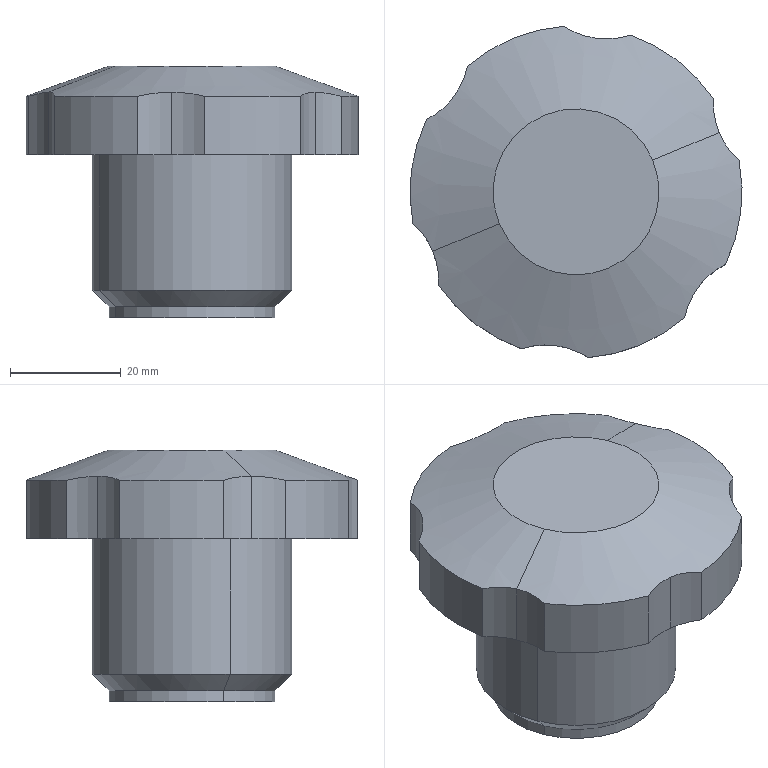Part | SolidWorks | features BaseBody 1 | 1 solid | 39 faces | box 60 x 59.84 x 45.5 mm | volume 53011 mm3 | cylinder 26 | plane 5 | cone 4 | torus 4 | commonest cylinder face diameters 28 x12 60 x6 20 x2 30 x2 36 x2 50 x2
STEP:
#1=CARTESIAN_POINT('',(32.407,459.424,549.15));
#2=VERTEX_POINT('',#1);
#3=CARTESIAN_POINT('',(78.593,478.576,549.15));
#4=VERTEX_POINT('',#3);
#5=CARTESIAN_POINT('',(55.5,469.,549.15));
#6=DIRECTION('',(0.,0.,1.));
#7=DIRECTION('',(-0.9237,-0.383,0.));
#8=AXIS2_PLACEMENT_3D('',#5,#6,#7);
#9=CIRCLE('',#8,25.);
#10=EDGE_CURVE('',#2,#4,#9,.T.);
#11=ORIENTED_EDGE('',*,*,#10,.T.);
#12=CARTESIAN_POINT('',(78.593,478.576,546.65));
#13=VERTEX_POINT('',#12);
#14=CARTESIAN_POINT('',(78.593,478.576,549.65));
#15=DIRECTION('',(0.,0.,-1.));
#16=VECTOR('',#15,1000.);
#17=LINE('',#14,#16);
#18=EDGE_CURVE('',#4,#13,#17,.T.);
#19=ORIENTED_EDGE('',*,*,#18,.T.);
#20=CARTESIAN_POINT('',(32.407,459.424,546.65));
#21=VERTEX_POINT('',#20);
#22=CARTESIAN_POINT('',(55.5,469.,546.65));
#23=DIRECTION('',(0.,0.,1.));
#24=DIRECTION('',(-0.9237,-0.383,0.));
#25=AXIS2_PLACEMENT_3D('',#22,#23,#24);
#26=CIRCLE('',#25,25.);
#27=EDGE_CURVE('',#21,#13,#26,.T.);
#28=ORIENTED_EDGE('',*,*,#27,.F.);
#29=CARTESIAN_POINT('',(32.407,459.424,549.65));
#30=DIRECTION('',(0.,0.,-1.));
#31=VECTOR('',#30,1000.);
#32=LINE('',#29,#31);
#33=EDGE_CURVE('',#2,#21,#32,.T.);
#34=ORIENTED_EDGE('',*,*,#33,.F.);
#35=EDGE_LOOP('',(#11,#19,#28,#34));
#36=FACE_OUTER_BOUND('',#35,.T.);
#37=CARTESIAN_POINT('',(55.5,469.,549.65));
#38=DIRECTION('',(0.,0.,-1.));
#39=DIRECTION('',(-0.9237,-0.383,0.));
#40=AXIS2_PLACEMENT_3D('',#37,#38,#39);
#41=CYLINDRICAL_SURFACE('',#40,25.);
#42=ADVANCED_FACE('',(#36),#41,.F.);
#43=CARTESIAN_POINT('',(38.873,462.105,549.15));
#44=VERTEX_POINT('',#43);
#45=CARTESIAN_POINT('',(72.127,475.895,549.15));
#46=VERTEX_POINT('',#45);
#47=CARTESIAN_POINT('',(55.5,469.,549.15));
#48=DIRECTION('',(0.,0.,-1.));
#49=DIRECTION('',(-0.9237,-0.383,0.));
#50=AXIS2_PLACEMENT_3D('',#47,#48,#49);
#51=CIRCLE('',#50,18.);
#52=EDGE_CURVE('',#44,#46,#51,.T.);
#53=ORIENTED_EDGE('',*,*,#52,.T.);
#54=CARTESIAN_POINT('',(72.127,475.895,522.15));
#55=VERTEX_POINT('',#54);
#56=CARTESIAN_POINT('',(72.127,475.895,549.65));
#57=DIRECTION('',(0.,0.,-1.));
#58=VECTOR('',#57,1000.);
#59=LINE('',#56,#58);
#60=EDGE_CURVE('',#46,#55,#59,.T.);
#61=ORIENTED_EDGE('',*,*,#60,.T.);
#62=CARTESIAN_POINT('',(38.873,462.105,522.15));
#63=VERTEX_POINT('',#62);
#64=CARTESIAN_POINT('',(55.5,469.,522.15));
#65=DIRECTION('',(0.,0.,1.));
#66=DIRECTION('',(0.9237,0.383,0.));
#67=AXIS2_PLACEMENT_3D('',#64,#65,#66);
#68=CIRCLE('',#67,18.);
#69=EDGE_CURVE('',#55,#63,#68,.T.);
#70=ORIENTED_EDGE('',*,*,#69,.T.);
#71=CARTESIAN_POINT('',(38.873,462.105,549.65));
#72=DIRECTION('',(0.,0.,-1.));
#73=VECTOR('',#72,1000.);
#74=LINE('',#71,#73);
#75=EDGE_CURVE('',#44,#63,#74,.T.);
#76=ORIENTED_EDGE('',*,*,#75,.F.);
#77=EDGE_LOOP('',(#53,#61,#70,#76));
#78=FACE_OUTER_BOUND('',#77,.T.);
#79=CARTESIAN_POINT('',(55.5,469.,549.65));
#80=DIRECTION('',(0.,0.,-1.));
#81=DIRECTION('',(-0.9237,-0.383,0.));
#82=AXIS2_PLACEMENT_3D('',#79,#80,#81);
#83=CYLINDRICAL_SURFACE('',#82,18.);
#84=ADVANCED_FACE('',(#78),#83,.T.);
#85=CARTESIAN_POINT('',(69.356,474.746,562.65));
#86=VERTEX_POINT('',#85);
#87=CARTESIAN_POINT('',(41.644,463.254,562.65));
#88=VERTEX_POINT('',#87);
#89=CARTESIAN_POINT('',(55.5,469.,562.65));
#90=DIRECTION('',(0.,0.,1.));
#91=DIRECTION('',(0.9237,0.383,0.));
#92=AXIS2_PLACEMENT_3D('',#89,#90,#91);
#93=CIRCLE('',#92,15.);
#94=EDGE_CURVE('',#86,#88,#93,.T.);
#95=ORIENTED_EDGE('',*,*,#94,.F.);
#96=CARTESIAN_POINT('',(81.364,479.725,557.918));
#97=VERTEX_POINT('',#96);
#98=CARTESIAN_POINT('',(83.212,480.491,557.19));
#99=DIRECTION('',(0.868,0.3599,-0.342));
#100=VECTOR('',#99,1000.);
#101=LINE('',#98,#100);
#102=EDGE_CURVE('',#86,#97,#101,.T.);
#103=ORIENTED_EDGE('',*,*,#102,.T.);
#104=CARTESIAN_POINT('',(80.318,485.855,557.19));
#105=VERTEX_POINT('',#104);
#106=CARTESIAN_POINT('',(80.318,485.855,557.19));
#107=CARTESIAN_POINT('',(80.261,484.818,557.419));
#108=CARTESIAN_POINT('',(80.318,483.785,557.601));
#109=CARTESIAN_POINT('',(80.536,482.496,557.757));
#110=CARTESIAN_POINT('',(80.587,482.239,557.785));
#111=CARTESIAN_POINT('',(80.704,481.724,557.833));
#112=CARTESIAN_POINT('',(80.77,481.467,557.854));
#113=CARTESIAN_POINT('',(80.99,480.705,557.902));
#114=CARTESIAN_POINT('',(81.164,480.21,557.918));
#115=CARTESIAN_POINT('',(81.364,479.725,557.918));
#116=B_SPLINE_CURVE_WITH_KNOTS('',3,(#106,#107,#108,#109,#110,#111,#112,#113,#114,#115),.UNSPECIFIED.,.F.,.F.,(4,2,2,2,4),(0.,0.003149,0.003936,0.004723,0.006297),.UNSPECIFIED.);
#117=EDGE_CURVE('',#105,#97,#116,.T.);
#118=ORIENTED_EDGE('',*,*,#117,.F.);
#119=CARTESIAN_POINT('',(65.335,497.342,557.19));
#120=VERTEX_POINT('',#119);
#121=CARTESIAN_POINT('',(55.5,469.,557.19));
#122=DIRECTION('',(0.,0.,-1.));
#123=DIRECTION('',(0.9237,0.383,0.));
#124=AXIS2_PLACEMENT_3D('',#121,#122,#123);
#125=CIRCLE('',#124,30.);
#126=EDGE_CURVE('',#120,#105,#125,.T.);
#127=ORIENTED_EDGE('',*,*,#126,.F.);
#128=CARTESIAN_POINT('',(59.144,496.762,557.918));
#129=VERTEX_POINT('',#128);
#130=CARTESIAN_POINT('',(59.144,496.762,557.918));
#131=CARTESIAN_POINT('',(59.663,496.694,557.918));
#132=CARTESIAN_POINT('',(60.186,496.655,557.902));
#133=CARTESIAN_POINT('',(61.239,496.636,557.838));
#134=CARTESIAN_POINT('',(61.771,496.656,557.789));
#135=CARTESIAN_POINT('',(63.335,496.805,557.601));
#136=CARTESIAN_POINT('',(64.349,497.018,557.419));
#137=CARTESIAN_POINT('',(65.335,497.342,557.19));
#138=B_SPLINE_CURVE_WITH_KNOTS('',3,(#130,#131,#132,#133,#134,#135,#136,#137),.UNSPECIFIED.,.F.,.F.,(4,2,2,4),(0.006297,0.007871,0.009445,0.01259),.UNSPECIFIED.);
#139=EDGE_CURVE('',#129,#120,#138,.T.);
#140=ORIENTED_EDGE('',*,*,#139,.F.);
#141=CARTESIAN_POINT('',(53.312,498.92,557.19));
#142=VERTEX_POINT('',#141);
#143=CARTESIAN_POINT('',(53.312,498.92,557.19));
#144=CARTESIAN_POINT('',(54.182,498.352,557.419));
#145=CARTESIAN_POINT('',(55.105,497.886,557.601));
#146=CARTESIAN_POINT('',(56.33,497.43,557.757));
#147=CARTESIAN_POINT('',(56.578,497.345,557.785));
#148=CARTESIAN_POINT('',(57.083,497.19,557.833));
#149=CARTESIAN_POINT('',(57.339,497.118,557.854));
#150=CARTESIAN_POINT('',(58.108,496.927,557.902));
#151=CARTESIAN_POINT('',(58.624,496.83,557.918));
#152=CARTESIAN_POINT('',(59.144,496.762,557.918));
#153=B_SPLINE_CURVE_WITH_KNOTS('',3,(#143,#144,#145,#146,#147,#148,#149,#150,#151,#152),.UNSPECIFIED.,.F.,.F.,(4,2,2,2,4),(0.,0.003149,0.003936,0.004723,0.006297),.UNSPECIFIED.);
#154=EDGE_CURVE('',#142,#129,#153,.T.);
#155=ORIENTED_EDGE('',*,*,#154,.F.);
#156=CARTESIAN_POINT('',(35.872,491.688,557.19));
#157=VERTEX_POINT('',#156);
#158=CARTESIAN_POINT('',(55.5,469.,557.19));
#159=DIRECTION('',(0.,0.,-1.));
#160=DIRECTION('',(0.9237,0.383,0.));
#161=AXIS2_PLACEMENT_3D('',#158,#159,#160);
#162=CIRCLE('',#161,30.);
#163=EDGE_CURVE('',#157,#142,#162,.T.);
#164=ORIENTED_EDGE('',*,*,#163,.F.);
#165=CARTESIAN_POINT('',(33.279,486.037,557.918));
#166=VERTEX_POINT('',#165);
#167=CARTESIAN_POINT('',(33.279,486.037,557.918));
#168=CARTESIAN_POINT('',(33.598,486.452,557.918));
#169=CARTESIAN_POINT('',(33.894,486.886,557.902));
#170=CARTESIAN_POINT('',(34.437,487.788,557.838));
#171=CARTESIAN_POINT('',(34.685,488.259,557.789));
#172=CARTESIAN_POINT('',(35.338,489.688,557.601));
#173=CARTESIAN_POINT('',(35.66,490.672,557.419));
#174=CARTESIAN_POINT('',(35.872,491.688,557.19));
#175=B_SPLINE_CURVE_WITH_KNOTS('',3,(#167,#168,#169,#170,#171,#172,#173,#174),.UNSPECIFIED.,.F.,.F.,(4,2,2,4),(0.006297,0.007871,0.009445,0.01259),.UNSPECIFIED.);
#176=EDGE_CURVE('',#166,#157,#175,.T.);
#177=ORIENTED_EDGE('',*,*,#176,.F.);
#178=CARTESIAN_POINT('',(28.494,482.065,557.19));
#179=VERTEX_POINT('',#178);
#180=CARTESIAN_POINT('',(28.494,482.065,557.19));
#181=CARTESIAN_POINT('',(29.421,482.534,557.419));
#182=CARTESIAN_POINT('',(30.287,483.101,557.601));
#183=CARTESIAN_POINT('',(31.294,483.934,557.757));
#184=CARTESIAN_POINT('',(31.491,484.107,557.785));
#185=CARTESIAN_POINT('',(31.878,484.465,557.833));
#186=CARTESIAN_POINT('',(32.068,484.652,557.854));
#187=CARTESIAN_POINT('',(32.618,485.222,557.902));
#188=CARTESIAN_POINT('',(32.96,485.621,557.918));
#189=CARTESIAN_POINT('',(33.279,486.037,557.918));
#190=B_SPLINE_CURVE_WITH_KNOTS('',3,(#180,#181,#182,#183,#184,#185,#186,#187,#188,#189),.UNSPECIFIED.,.F.,.F.,(4,2,2,2,4),(0.,0.003149,0.003936,0.004723,0.006297),.UNSPECIFIED.);
#191=EDGE_CURVE('',#179,#166,#190,.T.);
#192=ORIENTED_EDGE('',*,*,#191,.F.);
#193=CARTESIAN_POINT('',(26.038,463.346,557.19));
#194=VERTEX_POINT('',#193);
#195=CARTESIAN_POINT('',(55.5,469.,557.19));
#196=DIRECTION('',(0.,0.,-1.));
#197=DIRECTION('',(0.9237,0.383,0.));
#198=AXIS2_PLACEMENT_3D('',#195,#196,#197);
#199=CIRCLE('',#198,30.);
#200=EDGE_CURVE('',#194,#179,#199,.T.);
#201=ORIENTED_EDGE('',*,*,#200,.F.);
#202=CARTESIAN_POINT('',(29.636,458.275,557.918));
#203=VERTEX_POINT('',#202);
#204=CARTESIAN_POINT('',(29.636,458.275,557.918));
#205=CARTESIAN_POINT('',(29.435,458.759,557.918));
#206=CARTESIAN_POINT('',(29.207,459.231,557.902));
#207=CARTESIAN_POINT('',(28.697,460.153,557.838));
#208=CARTESIAN_POINT('',(28.413,460.603,557.789));
#209=CARTESIAN_POINT('',(27.502,461.883,557.601));
#210=CARTESIAN_POINT('',(26.811,462.654,557.419));
#211=CARTESIAN_POINT('',(26.038,463.346,557.19));
#212=B_SPLINE_CURVE_WITH_KNOTS('',3,(#204,#205,#206,#207,#208,#209,#210,#211),.UNSPECIFIED.,.F.,.F.,(4,2,2,4),(0.006297,0.007871,0.009445,0.01259),.UNSPECIFIED.);
#213=EDGE_CURVE('',#203,#194,#212,.T.);
#214=ORIENTED_EDGE('',*,*,#213,.F.);
#215=CARTESIAN_POINT('',(27.788,457.509,557.19));
#216=DIRECTION('',(-0.868,-0.3599,-0.342));
#217=VECTOR('',#216,1000.);
#218=LINE('',#215,#217);
#219=EDGE_CURVE('',#88,#203,#218,.T.);
#220=ORIENTED_EDGE('',*,*,#219,.F.);
#221=EDGE_LOOP('',(#95,#103,#118,#127,#140,#155,#164,#177,#192,#201,#214,#220));
#222=FACE_OUTER_BOUND('',#221,.T.);
#223=CARTESIAN_POINT('',(55.5,469.,557.19));
#224=DIRECTION('',(0.,0.,-1.));
#225=DIRECTION('',(-0.9237,-0.383,0.));
#226=AXIS2_PLACEMENT_3D('',#223,#224,#225);
#227=CONICAL_SURFACE('',#226,30.,1.222);
#228=ADVANCED_FACE('',(#222),#227,.T.);
#229=CARTESIAN_POINT('',(29.636,458.275,546.65));
#230=VERTEX_POINT('',#229);
#231=CARTESIAN_POINT('',(26.038,463.346,546.65));
#232=VERTEX_POINT('',#231);
#233=CARTESIAN_POINT('',(16.703,452.912,546.65));
#234=DIRECTION('',(0.,0.,1.));
#235=DIRECTION('',(-0.9237,-0.383,0.));
#236=AXIS2_PLACEMENT_3D('',#233,#234,#235);
#237=CIRCLE('',#236,14.);
#238=EDGE_CURVE('',#230,#232,#237,.T.);
#239=ORIENTED_EDGE('',*,*,#238,.F.);
#240=CARTESIAN_POINT('',(29.636,458.275,482.65));
#241=DIRECTION('',(0.,0.,1.));
#242=VECTOR('',#241,1000.);
#243=LINE('',#240,#242);
#244=EDGE_CURVE('',#230,#203,#243,.T.);
#245=ORIENTED_EDGE('',*,*,#244,.T.);
#246=ORIENTED_EDGE('',*,*,#213,.T.);
#247=CARTESIAN_POINT('',(26.038,463.346,551.92));
#248=DIRECTION('',(0.,0.,-1.));
#249=VECTOR('',#248,1000.);
#250=LINE('',#247,#249);
#251=EDGE_CURVE('',#194,#232,#250,.T.);
#252=ORIENTED_EDGE('',*,*,#251,.T.);
#253=EDGE_LOOP('',(#239,#245,#246,#252));
#254=FACE_OUTER_BOUND('',#253,.T.);
#255=CARTESIAN_POINT('',(16.703,452.912,482.65));
#256=DIRECTION('',(0.,0.,1.));
#257=DIRECTION('',(0.9237,0.383,0.));
#258=AXIS2_PLACEMENT_3D('',#255,#256,#257);
#259=CYLINDRICAL_SURFACE('',#258,14.);
#260=ADVANCED_FACE('',(#254),#259,.F.);
#261=CARTESIAN_POINT('',(51.856,441.238,546.65));
#262=VERTEX_POINT('',#261);
#263=CARTESIAN_POINT('',(45.665,440.658,546.65));
#264=VERTEX_POINT('',#263);
#265=CARTESIAN_POINT('',(50.034,427.357,546.65));
#266=DIRECTION('',(0.,0.,1.));
#267=DIRECTION('',(-0.9237,-0.383,0.));
#268=AXIS2_PLACEMENT_3D('',#265,#266,#267);
#269=CIRCLE('',#268,14.);
#270=EDGE_CURVE('',#262,#264,#269,.T.);
#271=ORIENTED_EDGE('',*,*,#270,.F.);
#272=CARTESIAN_POINT('',(51.856,441.238,557.918));
#273=VERTEX_POINT('',#272);
#274=CARTESIAN_POINT('',(51.856,441.238,482.65));
#275=DIRECTION('',(0.,0.,1.));
#276=VECTOR('',#275,1000.);
#277=LINE('',#274,#276);
#278=EDGE_CURVE('',#262,#273,#277,.T.);
#279=ORIENTED_EDGE('',*,*,#278,.T.);
#280=CARTESIAN_POINT('',(45.665,440.658,557.19));
#281=VERTEX_POINT('',#280);
#282=CARTESIAN_POINT('',(51.856,441.238,557.918));
#283=CARTESIAN_POINT('',(51.337,441.306,557.918));
#284=CARTESIAN_POINT('',(50.814,441.345,557.902));
#285=CARTESIAN_POINT('',(49.761,441.364,557.838));
#286=CARTESIAN_POINT('',(49.229,441.344,557.789));
#287=CARTESIAN_POINT('',(47.665,441.195,557.601));
#288=CARTESIAN_POINT('',(46.651,440.982,557.419));
#289=CARTESIAN_POINT('',(45.665,440.658,557.19));
#290=B_SPLINE_CURVE_WITH_KNOTS('',3,(#282,#283,#284,#285,#286,#287,#288,#289),.UNSPECIFIED.,.F.,.F.,(4,2,2,4),(0.006297,0.007871,0.009445,0.01259),.UNSPECIFIED.);
#291=EDGE_CURVE('',#273,#281,#290,.T.);
#292=ORIENTED_EDGE('',*,*,#291,.T.);
#293=CARTESIAN_POINT('',(45.665,440.658,551.92));
#294=DIRECTION('',(0.,0.,-1.));
#295=VECTOR('',#294,1000.);
#296=LINE('',#293,#295);
#297=EDGE_CURVE('',#281,#264,#296,.T.);
#298=ORIENTED_EDGE('',*,*,#297,.T.);
#299=EDGE_LOOP('',(#271,#279,#292,#298));
#300=FACE_OUTER_BOUND('',#299,.T.);
#301=CARTESIAN_POINT('',(50.034,427.357,482.65));
#302=DIRECTION('',(0.,0.,1.));
#303=DIRECTION('',(0.1301,0.9915,0.));
#304=AXIS2_PLACEMENT_3D('',#301,#302,#303);
#305=CYLINDRICAL_SURFACE('',#304,14.);
#306=ADVANCED_FACE('',(#300),#305,.F.);
#307=CARTESIAN_POINT('',(77.721,451.963,546.65));
#308=VERTEX_POINT('',#307);
#309=CARTESIAN_POINT('',(75.128,446.312,546.65));
#310=VERTEX_POINT('',#309);
#311=CARTESIAN_POINT('',(88.831,443.445,546.65));
#312=DIRECTION('',(0.,0.,1.));
#313=DIRECTION('',(-0.9237,-0.383,0.));
#314=AXIS2_PLACEMENT_3D('',#311,#312,#313);
#315=CIRCLE('',#314,14.);
#316=EDGE_CURVE('',#308,#310,#315,.T.);
#317=ORIENTED_EDGE('',*,*,#316,.F.);
#318=CARTESIAN_POINT('',(77.721,451.963,557.918));
#319=VERTEX_POINT('',#318);
#320=CARTESIAN_POINT('',(77.721,451.963,482.65));
#321=DIRECTION('',(0.,0.,1.));
#322=VECTOR('',#321,1000.);
#323=LINE('',#320,#322);
#324=EDGE_CURVE('',#308,#319,#323,.T.);
#325=ORIENTED_EDGE('',*,*,#324,.T.);
#326=CARTESIAN_POINT('',(75.128,446.312,557.19));
#327=VERTEX_POINT('',#326);
#328=CARTESIAN_POINT('',(77.721,451.963,557.918));
#329=CARTESIAN_POINT('',(77.402,451.548,557.918));
#330=CARTESIAN_POINT('',(77.106,451.114,557.902));
#331=CARTESIAN_POINT('',(76.563,450.212,557.838));
#332=CARTESIAN_POINT('',(76.315,449.741,557.789));
#333=CARTESIAN_POINT('',(75.662,448.312,557.601));
#334=CARTESIAN_POINT('',(75.34,447.328,557.419));
#335=CARTESIAN_POINT('',(75.128,446.312,557.19));
#336=B_SPLINE_CURVE_WITH_KNOTS('',3,(#328,#329,#330,#331,#332,#333,#334,#335),.UNSPECIFIED.,.F.,.F.,(4,2,2,4),(0.006297,0.007871,0.009445,0.01259),.UNSPECIFIED.);
#337=EDGE_CURVE('',#319,#327,#336,.T.);
#338=ORIENTED_EDGE('',*,*,#337,.T.);
#339=CARTESIAN_POINT('',(75.128,446.312,551.92));
#340=DIRECTION('',(0.,0.,-1.));
#341=VECTOR('',#340,1000.);
#342=LINE('',#339,#341);
#343=EDGE_CURVE('',#327,#310,#342,.T.);
#344=ORIENTED_EDGE('',*,*,#343,.T.);
#345=EDGE_LOOP('',(#317,#325,#338,#344));
#346=FACE_OUTER_BOUND('',#345,.T.);
#347=CARTESIAN_POINT('',(88.831,443.445,482.65));
#348=DIRECTION('',(0.,0.,1.));
#349=DIRECTION('',(-0.7936,0.6084,0.));
#350=AXIS2_PLACEMENT_3D('',#347,#348,#349);
#351=CYLINDRICAL_SURFACE('',#350,14.);
#352=ADVANCED_FACE('',(#346),#351,.F.);
#353=CARTESIAN_POINT('',(81.364,479.725,546.65));
#354=VERTEX_POINT('',#353);
#355=CARTESIAN_POINT('',(84.962,474.654,546.65));
#356=VERTEX_POINT('',#355);
#357=CARTESIAN_POINT('',(94.297,485.088,546.65));
#358=DIRECTION('',(0.,0.,1.));
#359=DIRECTION('',(-0.9237,-0.383,0.));
#360=AXIS2_PLACEMENT_3D('',#357,#358,#359);
#361=CIRCLE('',#360,14.);
#362=EDGE_CURVE('',#354,#356,#361,.T.);
#363=ORIENTED_EDGE('',*,*,#362,.F.);
#364=CARTESIAN_POINT('',(81.364,479.725,482.65));
#365=DIRECTION('',(0.,0.,1.));
#366=VECTOR('',#365,1000.);
#367=LINE('',#364,#366);
#368=EDGE_CURVE('',#354,#97,#367,.T.);
#369=ORIENTED_EDGE('',*,*,#368,.T.);
#370=CARTESIAN_POINT('',(84.962,474.654,557.19));
#371=VERTEX_POINT('',#370);
#372=CARTESIAN_POINT('',(81.364,479.725,557.918));
#373=CARTESIAN_POINT('',(81.565,479.241,557.918));
#374=CARTESIAN_POINT('',(81.793,478.769,557.902));
#375=CARTESIAN_POINT('',(82.303,477.847,557.838));
#376=CARTESIAN_POINT('',(82.587,477.397,557.789));
#377=CARTESIAN_POINT('',(83.498,476.117,557.601));
#378=CARTESIAN_POINT('',(84.189,475.346,557.419));
#379=CARTESIAN_POINT('',(84.962,474.654,557.19));
#380=B_SPLINE_CURVE_WITH_KNOTS('',3,(#372,#373,#374,#375,#376,#377,#378,#379),.UNSPECIFIED.,.F.,.F.,(4,2,2,4),(0.006297,0.007871,0.009445,0.01259),.UNSPECIFIED.);
#381=EDGE_CURVE('',#97,#371,#380,.T.);
#382=ORIENTED_EDGE('',*,*,#381,.T.);
#383=CARTESIAN_POINT('',(84.962,474.654,551.92));
#384=DIRECTION('',(0.,0.,-1.));
#385=VECTOR('',#384,1000.);
#386=LINE('',#383,#385);
#387=EDGE_CURVE('',#371,#356,#386,.T.);
#388=ORIENTED_EDGE('',*,*,#387,.T.);
#389=EDGE_LOOP('',(#363,#369,#382,#388));
#390=FACE_OUTER_BOUND('',#389,.T.);
#391=CARTESIAN_POINT('',(94.297,485.088,482.65));
#392=DIRECTION('',(0.,0.,1.));
#393=DIRECTION('',(-0.9237,-0.383,0.));
#394=AXIS2_PLACEMENT_3D('',#391,#392,#393);
#395=CYLINDRICAL_SURFACE('',#394,14.);
#396=ADVANCED_FACE('',(#390),#395,.F.);
#397=CARTESIAN_POINT('',(59.144,496.762,546.65));
#398=VERTEX_POINT('',#397);
#399=CARTESIAN_POINT('',(65.335,497.342,546.65));
#400=VERTEX_POINT('',#399);
#401=CARTESIAN_POINT('',(60.966,510.643,546.65));
#402=DIRECTION('',(0.,0.,1.));
#403=DIRECTION('',(-0.9237,-0.383,0.));
#404=AXIS2_PLACEMENT_3D('',#401,#402,#403);
#405=CIRCLE('',#404,14.);
#406=EDGE_CURVE('',#398,#400,#405,.T.);
#407=ORIENTED_EDGE('',*,*,#406,.F.);
#408=CARTESIAN_POINT('',(59.144,496.762,482.65));
#409=DIRECTION('',(0.,0.,1.));
#410=VECTOR('',#409,1000.);
#411=LINE('',#408,#410);
#412=EDGE_CURVE('',#398,#129,#411,.T.);
#413=ORIENTED_EDGE('',*,*,#412,.T.);
#414=ORIENTED_EDGE('',*,*,#139,.T.);
#415=CARTESIAN_POINT('',(65.335,497.342,551.92));
#416=DIRECTION('',(0.,0.,-1.));
#417=VECTOR('',#416,1000.);
#418=LINE('',#415,#417);
#419=EDGE_CURVE('',#120,#400,#418,.T.);
#420=ORIENTED_EDGE('',*,*,#419,.T.);
#421=EDGE_LOOP('',(#407,#413,#414,#420));
#422=FACE_OUTER_BOUND('',#421,.T.);
#423=CARTESIAN_POINT('',(60.966,510.643,482.65));
#424=DIRECTION('',(0.,0.,1.));
#425=DIRECTION('',(-0.1301,-0.9915,0.));
#426=AXIS2_PLACEMENT_3D('',#423,#424,#425);
#427=CYLINDRICAL_SURFACE('',#426,14.);
#428=ADVANCED_FACE('',(#422),#427,.F.);
#429=CARTESIAN_POINT('',(33.279,486.037,546.65));
#430=VERTEX_POINT('',#429);
#431=CARTESIAN_POINT('',(35.872,491.688,546.65));
#432=VERTEX_POINT('',#431);
#433=CARTESIAN_POINT('',(22.169,494.555,546.65));
#434=DIRECTION('',(0.,0.,1.));
#435=DIRECTION('',(-0.9237,-0.383,0.));
#436=AXIS2_PLACEMENT_3D('',#433,#434,#435);
#437=CIRCLE('',#436,14.);
#438=EDGE_CURVE('',#430,#432,#437,.T.);
#439=ORIENTED_EDGE('',*,*,#438,.F.);
#440=CARTESIAN_POINT('',(33.279,486.037,482.65));
#441=DIRECTION('',(0.,0.,1.));
#442=VECTOR('',#441,1000.);
#443=LINE('',#440,#442);
#444=EDGE_CURVE('',#430,#166,#443,.T.);
#445=ORIENTED_EDGE('',*,*,#444,.T.);
#446=ORIENTED_EDGE('',*,*,#176,.T.);
#447=CARTESIAN_POINT('',(35.872,491.688,551.92));
#448=DIRECTION('',(0.,0.,-1.));
#449=VECTOR('',#448,1000.);
#450=LINE('',#447,#449);
#451=EDGE_CURVE('',#157,#432,#450,.T.);
#452=ORIENTED_EDGE('',*,*,#451,.T.);
#453=EDGE_LOOP('',(#439,#445,#446,#452));
#454=FACE_OUTER_BOUND('',#453,.T.);
#455=CARTESIAN_POINT('',(22.169,494.555,482.65));
#456=DIRECTION('',(0.,0.,1.));
#457=DIRECTION('',(0.7936,-0.6084,0.));
#458=AXIS2_PLACEMENT_3D('',#455,#456,#457);
#459=CYLINDRICAL_SURFACE('',#458,14.);
#460=ADVANCED_FACE('',(#454),#459,.F.);
#461=CARTESIAN_POINT('',(78.131,478.385,549.65));
#462=VERTEX_POINT('',#461);
#463=CARTESIAN_POINT('',(32.869,459.615,549.65));
#464=VERTEX_POINT('',#463);
#465=CARTESIAN_POINT('',(55.5,469.,549.65));
#466=DIRECTION('',(0.,0.,-1.));
#467=DIRECTION('',(-0.9237,-0.383,0.));
#468=AXIS2_PLACEMENT_3D('',#465,#466,#467);
#469=CIRCLE('',#468,24.5);
#470=EDGE_CURVE('',#462,#464,#469,.T.);
#471=ORIENTED_EDGE('',*,*,#470,.F.);
#472=CARTESIAN_POINT('',(78.131,478.385,549.15));
#473=DIRECTION('',(-0.383,0.9237,0.));
#474=DIRECTION('',(-0.9237,-0.383,0.));
#475=AXIS2_PLACEMENT_3D('',#472,#473,#474);
#476=CIRCLE('',#475,0.5);
#477=EDGE_CURVE('',#462,#4,#476,.T.);
#478=ORIENTED_EDGE('',*,*,#477,.T.);
#479=ORIENTED_EDGE('',*,*,#10,.F.);
#480=CARTESIAN_POINT('',(32.869,459.615,549.15));
#481=DIRECTION('',(0.383,-0.9237,0.));
#482=DIRECTION('',(0.9237,0.383,0.));
#483=AXIS2_PLACEMENT_3D('',#480,#481,#482);
#484=CIRCLE('',#483,0.5);
#485=EDGE_CURVE('',#464,#2,#484,.T.);
#486=ORIENTED_EDGE('',*,*,#485,.F.);
#487=EDGE_LOOP('',(#471,#478,#479,#486));
#488=FACE_OUTER_BOUND('',#487,.T.);
#489=CARTESIAN_POINT('',(55.5,469.,549.15));
#490=DIRECTION('',(0.,0.,-1.));
#491=DIRECTION('',(-0.9237,-0.383,0.));
#492=AXIS2_PLACEMENT_3D('',#489,#490,#491);
#493=TOROIDAL_SURFACE('',#492,24.5,0.5);
#494=ADVANCED_FACE('',(#488),#493,.F.);
#495=CARTESIAN_POINT('',(55.5,469.,549.15));
#496=DIRECTION('',(0.,0.,-1.));
#497=DIRECTION('',(-0.9237,-0.383,0.));
#498=AXIS2_PLACEMENT_3D('',#495,#496,#497);
#499=CIRCLE('',#498,18.);
#500=EDGE_CURVE('',#46,#44,#499,.T.);
#501=ORIENTED_EDGE('',*,*,#500,.F.);
#502=CARTESIAN_POINT('',(72.589,476.086,549.65));
#503=VERTEX_POINT('',#502);
#504=CARTESIAN_POINT('',(72.589,476.086,549.15));
#505=DIRECTION('',(-0.383,0.9237,0.));
#506=DIRECTION('',(-0.9237,-0.383,0.));
#507=AXIS2_PLACEMENT_3D('',#504,#505,#506);
#508=CIRCLE('',#507,0.5);
#509=EDGE_CURVE('',#46,#503,#508,.T.);
#510=ORIENTED_EDGE('',*,*,#509,.T.);
#511=CARTESIAN_POINT('',(38.411,461.914,549.65));
#512=VERTEX_POINT('',#511);
#513=CARTESIAN_POINT('',(55.5,469.,549.65));
#514=DIRECTION('',(0.,0.,1.));
#515=DIRECTION('',(-0.9237,-0.383,0.));
#516=AXIS2_PLACEMENT_3D('',#513,#514,#515);
#517=CIRCLE('',#516,18.5);
#518=EDGE_CURVE('',#512,#503,#517,.T.);
#519=ORIENTED_EDGE('',*,*,#518,.F.);
#520=CARTESIAN_POINT('',(38.411,461.914,549.15));
#521=DIRECTION('',(0.383,-0.9237,0.));
#522=DIRECTION('',(0.9237,0.383,0.));
#523=AXIS2_PLACEMENT_3D('',#520,#521,#522);
#524=CIRCLE('',#523,0.5);
#525=EDGE_CURVE('',#44,#512,#524,.T.);
#526=ORIENTED_EDGE('',*,*,#525,.F.);
#527=EDGE_LOOP('',(#501,#510,#519,#526));
#528=FACE_OUTER_BOUND('',#527,.T.);
#529=CARTESIAN_POINT('',(55.5,469.,549.15));
#530=DIRECTION('',(0.,0.,-1.));
#531=DIRECTION('',(-0.9237,-0.383,0.));
#532=AXIS2_PLACEMENT_3D('',#529,#530,#531);
#533=TOROIDAL_SURFACE('',#532,18.5,0.5);
#534=ADVANCED_FACE('',(#528),#533,.F.);
#535=CARTESIAN_POINT('',(69.356,474.746,517.15));
#536=VERTEX_POINT('',#535);
#537=CARTESIAN_POINT('',(41.644,463.254,517.15));
#538=VERTEX_POINT('',#537);
#539=CARTESIAN_POINT('',(55.5,469.,517.15));
#540=DIRECTION('',(0.,0.,1.));
#541=DIRECTION('',(0.9237,0.383,0.));
#542=AXIS2_PLACEMENT_3D('',#539,#540,#541);
#543=CIRCLE('',#542,15.);
#544=EDGE_CURVE('',#536,#538,#543,.T.);
#545=ORIENTED_EDGE('',*,*,#544,.T.);
#546=CARTESIAN_POINT('',(41.644,463.254,519.15));
#547=VERTEX_POINT('',#546);
#548=CARTESIAN_POINT('',(41.644,463.254,517.15));
#549=DIRECTION('',(0.,0.,1.));
#550=VECTOR('',#549,1000.);
#551=LINE('',#548,#550);
#552=EDGE_CURVE('',#538,#547,#551,.T.);
#553=ORIENTED_EDGE('',*,*,#552,.T.);
#554=CARTESIAN_POINT('',(69.356,474.746,519.15));
#555=VERTEX_POINT('',#554);
#556=CARTESIAN_POINT('',(55.5,469.,519.15));
#557=DIRECTION('',(0.,0.,1.));
#558=DIRECTION('',(0.9237,0.383,0.));
#559=AXIS2_PLACEMENT_3D('',#556,#557,#558);
#560=CIRCLE('',#559,15.);
#561=EDGE_CURVE('',#555,#547,#560,.T.);
#562=ORIENTED_EDGE('',*,*,#561,.F.);
#563=CARTESIAN_POINT('',(69.356,474.746,517.15));
#564=DIRECTION('',(0.,0.,1.));
#565=VECTOR('',#564,1000.);
#566=LINE('',#563,#565);
#567=EDGE_CURVE('',#536,#555,#566,.T.);
#568=ORIENTED_EDGE('',*,*,#567,.F.);
#569=EDGE_LOOP('',(#545,#553,#562,#568));
#570=FACE_OUTER_BOUND('',#569,.T.);
#571=CARTESIAN_POINT('',(55.5,469.,517.15));
#572=DIRECTION('',(0.,0.,1.));
#573=DIRECTION('',(0.9237,0.383,0.));
#574=AXIS2_PLACEMENT_3D('',#571,#572,#573);
#575=CYLINDRICAL_SURFACE('',#574,15.);
#576=ADVANCED_FACE('',(#570),#575,.T.);
#577=CARTESIAN_POINT('',(46.263,465.17,517.15));
#578=VERTEX_POINT('',#577);
#579=CARTESIAN_POINT('',(64.737,472.83,517.15));
#580=VERTEX_POINT('',#579);
#581=CARTESIAN_POINT('',(55.5,469.,517.15));
#582=DIRECTION('',(0.,0.,1.));
#583=DIRECTION('',(0.9237,0.383,0.));
#584=AXIS2_PLACEMENT_3D('',#581,#582,#583);
#585=CIRCLE('',#584,10.);
#586=EDGE_CURVE('',#578,#580,#585,.T.);
#587=ORIENTED_EDGE('',*,*,#586,.F.);
#588=CARTESIAN_POINT('',(46.263,465.17,551.65));
#589=VERTEX_POINT('',#588);
#590=CARTESIAN_POINT('',(46.263,465.17,517.15));
#591=DIRECTION('',(0.,0.,1.));
#592=VECTOR('',#591,1000.);
#593=LINE('',#590,#592);
#594=EDGE_CURVE('',#578,#589,#593,.T.);
#595=ORIENTED_EDGE('',*,*,#594,.T.);
#596=CARTESIAN_POINT('',(64.737,472.83,551.65));
#597=VERTEX_POINT('',#596);
#598=CARTESIAN_POINT('',(55.5,469.,551.65));
#599=DIRECTION('',(0.,0.,1.));
#600=DIRECTION('',(0.9237,0.383,0.));
#601=AXIS2_PLACEMENT_3D('',#598,#599,#600);
#602=CIRCLE('',#601,10.);
#603=EDGE_CURVE('',#589,#597,#602,.T.);
#604=ORIENTED_EDGE('',*,*,#603,.T.);
#605=CARTESIAN_POINT('',(64.737,472.83,517.15));
#606=DIRECTION('',(0.,0.,1.));
#607=VECTOR('',#606,1000.);
#608=LINE('',#605,#607);
#609=EDGE_CURVE('',#580,#597,#608,.T.);
#610=ORIENTED_EDGE('',*,*,#609,.F.);
#611=EDGE_LOOP('',(#587,#595,#604,#610));
#612=FACE_OUTER_BOUND('',#611,.T.);
#613=CARTESIAN_POINT('',(55.5,469.,517.15));
#614=DIRECTION('',(0.,0.,1.));
#615=DIRECTION('',(0.9237,0.383,0.));
#616=AXIS2_PLACEMENT_3D('',#613,#614,#615);
#617=CYLINDRICAL_SURFACE('',#616,10.);
#618=ADVANCED_FACE('',(#612),#617,.F.);
#619=ORIENTED_EDGE('',*,*,#561,.T.);
#620=CARTESIAN_POINT('',(38.873,462.105,522.15));
#621=DIRECTION('',(-0.6532,-0.2709,0.7071));
#622=VECTOR('',#621,1000.);
#623=LINE('',#620,#622);
#624=EDGE_CURVE('',#547,#63,#623,.T.);
#625=ORIENTED_EDGE('',*,*,#624,.T.);
#626=ORIENTED_EDGE('',*,*,#69,.F.);
#627=CARTESIAN_POINT('',(72.127,475.895,522.15));
#628=DIRECTION('',(0.6532,0.2709,0.7071));
#629=VECTOR('',#628,1000.);
#630=LINE('',#627,#629);
#631=EDGE_CURVE('',#555,#55,#630,.T.);
#632=ORIENTED_EDGE('',*,*,#631,.F.);
#633=EDGE_LOOP('',(#619,#625,#626,#632));
#634=FACE_OUTER_BOUND('',#633,.T.);
#635=CARTESIAN_POINT('',(55.5,469.,522.15));
#636=DIRECTION('',(0.,0.,1.));
#637=DIRECTION('',(0.9237,0.383,0.));
#638=AXIS2_PLACEMENT_3D('',#635,#636,#637);
#639=CONICAL_SURFACE('',#638,18.,0.7854);
#640=ADVANCED_FACE('',(#634),#639,.T.);
#641=ORIENTED_EDGE('',*,*,#624,.F.);
#642=CARTESIAN_POINT('',(55.5,469.,519.15));
#643=DIRECTION('',(0.,0.,1.));
#644=DIRECTION('',(0.9237,0.383,0.));
#645=AXIS2_PLACEMENT_3D('',#642,#643,#644);
#646=CIRCLE('',#645,15.);
#647=EDGE_CURVE('',#547,#555,#646,.T.);
#648=ORIENTED_EDGE('',*,*,#647,.T.);
#649=ORIENTED_EDGE('',*,*,#631,.T.);
#650=CARTESIAN_POINT('',(55.5,469.,522.15));
#651=DIRECTION('',(0.,0.,1.));
#652=DIRECTION('',(0.9237,0.383,0.));
#653=AXIS2_PLACEMENT_3D('',#650,#651,#652);
#654=CIRCLE('',#653,18.);
#655=EDGE_CURVE('',#63,#55,#654,.T.);
#656=ORIENTED_EDGE('',*,*,#655,.F.);
#657=EDGE_LOOP('',(#641,#648,#649,#656));
#658=FACE_OUTER_BOUND('',#657,.T.);
#659=CARTESIAN_POINT('',(55.5,469.,522.15));
#660=DIRECTION('',(0.,0.,1.));
#661=DIRECTION('',(0.9237,0.383,0.));
#662=AXIS2_PLACEMENT_3D('',#659,#660,#661);
#663=CONICAL_SURFACE('',#662,18.,0.7854);
#664=ADVANCED_FACE('',(#658),#663,.T.);
#665=ORIENTED_EDGE('',*,*,#544,.F.);
#666=CARTESIAN_POINT('',(55.5,469.,517.15));
#667=DIRECTION('',(0.,0.,1.));
#668=DIRECTION('',(0.9237,0.383,0.));
#669=AXIS2_PLACEMENT_3D('',#666,#667,#668);
#670=CIRCLE('',#669,15.);
#671=EDGE_CURVE('',#538,#536,#670,.T.);
#672=ORIENTED_EDGE('',*,*,#671,.F.);
#673=EDGE_LOOP('',(#665,#672));
#674=FACE_OUTER_BOUND('',#673,.T.);
#675=CARTESIAN_POINT('',(55.5,469.,517.15));
#676=DIRECTION('',(0.,0.,1.));
#677=DIRECTION('',(0.9237,0.383,0.));
#678=AXIS2_PLACEMENT_3D('',#675,#676,#677);
#679=CIRCLE('',#678,10.);
#680=EDGE_CURVE('',#580,#578,#679,.T.);
#681=ORIENTED_EDGE('',*,*,#680,.T.);
#682=ORIENTED_EDGE('',*,*,#586,.T.);
#683=EDGE_LOOP('',(#681,#682));
#684=FACE_BOUND('',#683,.T.);
#685=CARTESIAN_POINT('',(55.5,469.,517.15));
#686=DIRECTION('',(0.,0.,-1.));
#687=DIRECTION('',(0.,-1.,0.));
#688=AXIS2_PLACEMENT_3D('',#685,#686,#687);
#689=PLANE('',#688);
#690=ADVANCED_FACE('',(#674,#684),#689,.T.);
#691=ORIENTED_EDGE('',*,*,#594,.F.);
#692=ORIENTED_EDGE('',*,*,#680,.F.);
#693=ORIENTED_EDGE('',*,*,#609,.T.);
#694=CARTESIAN_POINT('',(55.5,469.,551.65));
#695=DIRECTION('',(0.,0.,1.));
#696=DIRECTION('',(0.9237,0.383,0.));
#697=AXIS2_PLACEMENT_3D('',#694,#695,#696);
#698=CIRCLE('',#697,10.);
#699=EDGE_CURVE('',#597,#589,#698,.T.);
#700=ORIENTED_EDGE('',*,*,#699,.T.);
#701=EDGE_LOOP('',(#691,#692,#693,#700));
#702=FACE_OUTER_BOUND('',#701,.T.);
#703=CARTESIAN_POINT('',(55.5,469.,517.15));
#704=DIRECTION('',(0.,0.,1.));
#705=DIRECTION('',(0.9237,0.383,0.));
#706=AXIS2_PLACEMENT_3D('',#703,#704,#705);
#707=CYLINDRICAL_SURFACE('',#706,10.);
#708=ADVANCED_FACE('',(#702),#707,.F.);
#709=ORIENTED_EDGE('',*,*,#699,.F.);
#710=ORIENTED_EDGE('',*,*,#603,.F.);
#711=EDGE_LOOP('',(#709,#710));
#712=FACE_OUTER_BOUND('',#711,.T.);
#713=CARTESIAN_POINT('',(55.5,469.,551.65));
#714=DIRECTION('',(0.,0.,1.));
#715=DIRECTION('',(1.,0.,0.));
#716=AXIS2_PLACEMENT_3D('',#713,#714,#715);
#717=PLANE('',#716);
#718=ADVANCED_FACE('',(#712),#717,.F.);
#719=ORIENTED_EDGE('',*,*,#552,.F.);
#720=ORIENTED_EDGE('',*,*,#671,.T.);
#721=ORIENTED_EDGE('',*,*,#567,.T.);
#722=ORIENTED_EDGE('',*,*,#647,.F.);
#723=EDGE_LOOP('',(#719,#720,#721,#722));
#724=FACE_OUTER_BOUND('',#723,.T.);
#725=CARTESIAN_POINT('',(55.5,469.,517.15));
#726=DIRECTION('',(0.,0.,1.));
#727=DIRECTION('',(0.9237,0.383,0.));
#728=AXIS2_PLACEMENT_3D('',#725,#726,#727);
#729=CYLINDRICAL_SURFACE('',#728,15.);
#730=ADVANCED_FACE('',(#724),#729,.T.);
#731=ORIENTED_EDGE('',*,*,#509,.F.);
#732=ORIENTED_EDGE('',*,*,#52,.F.);
#733=ORIENTED_EDGE('',*,*,#525,.T.);
#734=CARTESIAN_POINT('',(55.5,469.,549.65));
#735=DIRECTION('',(0.,0.,1.));
#736=DIRECTION('',(-0.9237,-0.383,0.));
#737=AXIS2_PLACEMENT_3D('',#734,#735,#736);
#738=CIRCLE('',#737,18.5);
#739=EDGE_CURVE('',#503,#512,#738,.T.);
#740=ORIENTED_EDGE('',*,*,#739,.F.);
#741=EDGE_LOOP('',(#731,#732,#733,#740));
#742=FACE_OUTER_BOUND('',#741,.T.);
#743=CARTESIAN_POINT('',(55.5,469.,549.15));
#744=DIRECTION('',(0.,0.,-1.));
#745=DIRECTION('',(-0.9237,-0.383,0.));
#746=AXIS2_PLACEMENT_3D('',#743,#744,#745);
#747=TOROIDAL_SURFACE('',#746,18.5,0.5);
#748=ADVANCED_FACE('',(#742),#747,.F.);
#749=ORIENTED_EDGE('',*,*,#477,.F.);
#750=CARTESIAN_POINT('',(55.5,469.,549.65));
#751=DIRECTION('',(0.,0.,-1.));
#752=DIRECTION('',(-0.9237,-0.383,0.));
#753=AXIS2_PLACEMENT_3D('',#750,#751,#752);
#754=CIRCLE('',#753,24.5);
#755=EDGE_CURVE('',#464,#462,#754,.T.);
#756=ORIENTED_EDGE('',*,*,#755,.F.);
#757=ORIENTED_EDGE('',*,*,#485,.T.);
#758=CARTESIAN_POINT('',(55.5,469.,549.15));
#759=DIRECTION('',(0.,0.,1.));
#760=DIRECTION('',(-0.9237,-0.383,0.));
#761=AXIS2_PLACEMENT_3D('',#758,#759,#760);
#762=CIRCLE('',#761,25.);
#763=EDGE_CURVE('',#4,#2,#762,.T.);
#764=ORIENTED_EDGE('',*,*,#763,.F.);
#765=EDGE_LOOP('',(#749,#756,#757,#764));
#766=FACE_OUTER_BOUND('',#765,.T.);
#767=CARTESIAN_POINT('',(55.5,469.,549.15));
#768=DIRECTION('',(0.,0.,-1.));
#769=DIRECTION('',(-0.9237,-0.383,0.));
#770=AXIS2_PLACEMENT_3D('',#767,#768,#769);
#771=TOROIDAL_SURFACE('',#770,24.5,0.5);
#772=ADVANCED_FACE('',(#766),#771,.F.);
#773=ORIENTED_EDGE('',*,*,#444,.F.);
#774=CARTESIAN_POINT('',(28.494,482.065,546.65));
#775=VERTEX_POINT('',#774);
#776=CARTESIAN_POINT('',(22.169,494.555,546.65));
#777=DIRECTION('',(0.,0.,1.));
#778=DIRECTION('',(-0.9237,-0.383,0.));
#779=AXIS2_PLACEMENT_3D('',#776,#777,#778);
#780=CIRCLE('',#779,14.);
#781=EDGE_CURVE('',#775,#430,#780,.T.);
#782=ORIENTED_EDGE('',*,*,#781,.F.);
#783=CARTESIAN_POINT('',(28.494,482.065,551.92));
#784=DIRECTION('',(0.,0.,1.));
#785=VECTOR('',#784,1000.);
#786=LINE('',#783,#785);
#787=EDGE_CURVE('',#775,#179,#786,.T.);
#788=ORIENTED_EDGE('',*,*,#787,.T.);
#789=ORIENTED_EDGE('',*,*,#191,.T.);
#790=EDGE_LOOP('',(#773,#782,#788,#789));
#791=FACE_OUTER_BOUND('',#790,.T.);
#792=CARTESIAN_POINT('',(22.169,494.555,482.65));
#793=DIRECTION('',(0.,0.,1.));
#794=DIRECTION('',(0.7936,-0.6084,0.));
#795=AXIS2_PLACEMENT_3D('',#792,#793,#794);
#796=CYLINDRICAL_SURFACE('',#795,14.);
#797=ADVANCED_FACE('',(#791),#796,.F.);
#798=ORIENTED_EDGE('',*,*,#412,.F.);
#799=CARTESIAN_POINT('',(53.312,498.92,546.65));
#800=VERTEX_POINT('',#799);
#801=CARTESIAN_POINT('',(60.966,510.643,546.65));
#802=DIRECTION('',(0.,0.,1.));
#803=DIRECTION('',(-0.9237,-0.383,0.));
#804=AXIS2_PLACEMENT_3D('',#801,#802,#803);
#805=CIRCLE('',#804,14.);
#806=EDGE_CURVE('',#800,#398,#805,.T.);
#807=ORIENTED_EDGE('',*,*,#806,.F.);
#808=CARTESIAN_POINT('',(53.312,498.92,551.92));
#809=DIRECTION('',(0.,0.,1.));
#810=VECTOR('',#809,1000.);
#811=LINE('',#808,#810);
#812=EDGE_CURVE('',#800,#142,#811,.T.);
#813=ORIENTED_EDGE('',*,*,#812,.T.);
#814=ORIENTED_EDGE('',*,*,#154,.T.);
#815=EDGE_LOOP('',(#798,#807,#813,#814));
#816=FACE_OUTER_BOUND('',#815,.T.);
#817=CARTESIAN_POINT('',(60.966,510.643,482.65));
#818=DIRECTION('',(0.,0.,1.));
#819=DIRECTION('',(-0.1301,-0.9915,0.));
#820=AXIS2_PLACEMENT_3D('',#817,#818,#819);
#821=CYLINDRICAL_SURFACE('',#820,14.);
#822=ADVANCED_FACE('',(#816),#821,.F.);
#823=ORIENTED_EDGE('',*,*,#368,.F.);
#824=CARTESIAN_POINT('',(80.318,485.855,546.65));
#825=VERTEX_POINT('',#824);
#826=CARTESIAN_POINT('',(94.297,485.088,546.65));
#827=DIRECTION('',(0.,0.,1.));
#828=DIRECTION('',(-0.9237,-0.383,0.));
#829=AXIS2_PLACEMENT_3D('',#826,#827,#828);
#830=CIRCLE('',#829,14.);
#831=EDGE_CURVE('',#825,#354,#830,.T.);
#832=ORIENTED_EDGE('',*,*,#831,.F.);
#833=CARTESIAN_POINT('',(80.318,485.855,551.92));
#834=DIRECTION('',(0.,0.,1.));
#835=VECTOR('',#834,1000.);
#836=LINE('',#833,#835);
#837=EDGE_CURVE('',#825,#105,#836,.T.);
#838=ORIENTED_EDGE('',*,*,#837,.T.);
#839=ORIENTED_EDGE('',*,*,#117,.T.);
#840=EDGE_LOOP('',(#823,#832,#838,#839));
#841=FACE_OUTER_BOUND('',#840,.T.);
#842=CARTESIAN_POINT('',(94.297,485.088,482.65));
#843=DIRECTION('',(0.,0.,1.));
#844=DIRECTION('',(-0.9237,-0.383,0.));
#845=AXIS2_PLACEMENT_3D('',#842,#843,#844);
#846=CYLINDRICAL_SURFACE('',#845,14.);
#847=ADVANCED_FACE('',(#841),#846,.F.);
#848=ORIENTED_EDGE('',*,*,#324,.F.);
#849=CARTESIAN_POINT('',(82.506,455.935,546.65));
#850=VERTEX_POINT('',#849);
#851=CARTESIAN_POINT('',(88.831,443.445,546.65));
#852=DIRECTION('',(0.,0.,1.));
#853=DIRECTION('',(-0.9237,-0.383,0.));
#854=AXIS2_PLACEMENT_3D('',#851,#852,#853);
#855=CIRCLE('',#854,14.);
#856=EDGE_CURVE('',#850,#308,#855,.T.);
#857=ORIENTED_EDGE('',*,*,#856,.F.);
#858=CARTESIAN_POINT('',(82.506,455.935,557.19));
#859=VERTEX_POINT('',#858);
#860=CARTESIAN_POINT('',(82.506,455.935,551.92));
#861=DIRECTION('',(0.,0.,1.));
#862=VECTOR('',#861,1000.);
#863=LINE('',#860,#862);
#864=EDGE_CURVE('',#850,#859,#863,.T.);
#865=ORIENTED_EDGE('',*,*,#864,.T.);
#866=CARTESIAN_POINT('',(82.506,455.935,557.19));
#867=CARTESIAN_POINT('',(81.579,455.466,557.419));
#868=CARTESIAN_POINT('',(80.713,454.899,557.601));
#869=CARTESIAN_POINT('',(79.706,454.066,557.757));
#870=CARTESIAN_POINT('',(79.509,453.893,557.785));
#871=CARTESIAN_POINT('',(79.122,453.535,557.833));
#872=CARTESIAN_POINT('',(78.932,453.348,557.854));
#873=CARTESIAN_POINT('',(78.382,452.778,557.902));
#874=CARTESIAN_POINT('',(78.04,452.379,557.918));
#875=CARTESIAN_POINT('',(77.721,451.963,557.918));
#876=B_SPLINE_CURVE_WITH_KNOTS('',3,(#866,#867,#868,#869,#870,#871,#872,#873,#874,#875),.UNSPECIFIED.,.F.,.F.,(4,2,2,2,4),(0.,0.003149,0.003936,0.004723,0.006297),.UNSPECIFIED.);
#877=EDGE_CURVE('',#859,#319,#876,.T.);
#878=ORIENTED_EDGE('',*,*,#877,.T.);
#879=EDGE_LOOP('',(#848,#857,#865,#878));
#880=FACE_OUTER_BOUND('',#879,.T.);
#881=CARTESIAN_POINT('',(88.831,443.445,482.65));
#882=DIRECTION('',(0.,0.,1.));
#883=DIRECTION('',(-0.7936,0.6084,0.));
#884=AXIS2_PLACEMENT_3D('',#881,#882,#883);
#885=CYLINDRICAL_SURFACE('',#884,14.);
#886=ADVANCED_FACE('',(#880),#885,.F.);
#887=ORIENTED_EDGE('',*,*,#278,.F.);
#888=CARTESIAN_POINT('',(57.688,439.08,546.65));
#889=VERTEX_POINT('',#888);
#890=CARTESIAN_POINT('',(50.034,427.357,546.65));
#891=DIRECTION('',(0.,0.,1.));
#892=DIRECTION('',(-0.9237,-0.383,0.));
#893=AXIS2_PLACEMENT_3D('',#890,#891,#892);
#894=CIRCLE('',#893,14.);
#895=EDGE_CURVE('',#889,#262,#894,.T.);
#896=ORIENTED_EDGE('',*,*,#895,.F.);
#897=CARTESIAN_POINT('',(57.688,439.08,557.19));
#898=VERTEX_POINT('',#897);
#899=CARTESIAN_POINT('',(57.688,439.08,551.92));
#900=DIRECTION('',(0.,0.,1.));
#901=VECTOR('',#900,1000.);
#902=LINE('',#899,#901);
#903=EDGE_CURVE('',#889,#898,#902,.T.);
#904=ORIENTED_EDGE('',*,*,#903,.T.);
#905=CARTESIAN_POINT('',(57.688,439.08,557.19));
#906=CARTESIAN_POINT('',(56.818,439.648,557.419));
#907=CARTESIAN_POINT('',(55.895,440.114,557.601));
#908=CARTESIAN_POINT('',(54.67,440.57,557.757));
#909=CARTESIAN_POINT('',(54.422,440.655,557.785));
#910=CARTESIAN_POINT('',(53.917,440.81,557.833));
#911=CARTESIAN_POINT('',(53.661,440.882,557.854));
#912=CARTESIAN_POINT('',(52.892,441.073,557.902));
#913=CARTESIAN_POINT('',(52.376,441.17,557.918));
#914=CARTESIAN_POINT('',(51.856,441.238,557.918));
#915=B_SPLINE_CURVE_WITH_KNOTS('',3,(#905,#906,#907,#908,#909,#910,#911,#912,#913,#914),.UNSPECIFIED.,.F.,.F.,(4,2,2,2,4),(0.,0.003149,0.003936,0.004723,0.006297),.UNSPECIFIED.);
#916=EDGE_CURVE('',#898,#273,#915,.T.);
#917=ORIENTED_EDGE('',*,*,#916,.T.);
#918=EDGE_LOOP('',(#887,#896,#904,#917));
#919=FACE_OUTER_BOUND('',#918,.T.);
#920=CARTESIAN_POINT('',(50.034,427.357,482.65));
#921=DIRECTION('',(0.,0.,1.));
#922=DIRECTION('',(0.1301,0.9915,0.));
#923=AXIS2_PLACEMENT_3D('',#920,#921,#922);
#924=CYLINDRICAL_SURFACE('',#923,14.);
#925=ADVANCED_FACE('',(#919),#924,.F.);
#926=ORIENTED_EDGE('',*,*,#244,.F.);
#927=CARTESIAN_POINT('',(30.682,452.145,546.65));
#928=VERTEX_POINT('',#927);
#929=CARTESIAN_POINT('',(16.703,452.912,546.65));
#930=DIRECTION('',(0.,0.,1.));
#931=DIRECTION('',(-0.9237,-0.383,0.));
#932=AXIS2_PLACEMENT_3D('',#929,#930,#931);
#933=CIRCLE('',#932,14.);
#934=EDGE_CURVE('',#928,#230,#933,.T.);
#935=ORIENTED_EDGE('',*,*,#934,.F.);
#936=CARTESIAN_POINT('',(30.682,452.145,557.19));
#937=VERTEX_POINT('',#936);
#938=CARTESIAN_POINT('',(30.682,452.145,551.92));
#939=DIRECTION('',(0.,0.,1.));
#940=VECTOR('',#939,1000.);
#941=LINE('',#938,#940);
#942=EDGE_CURVE('',#928,#937,#941,.T.);
#943=ORIENTED_EDGE('',*,*,#942,.T.);
#944=CARTESIAN_POINT('',(30.682,452.145,557.19));
#945=CARTESIAN_POINT('',(30.739,453.182,557.419));
#946=CARTESIAN_POINT('',(30.682,454.215,557.601));
#947=CARTESIAN_POINT('',(30.464,455.504,557.757));
#948=CARTESIAN_POINT('',(30.413,455.761,557.785));
#949=CARTESIAN_POINT('',(30.296,456.276,557.833));
#950=CARTESIAN_POINT('',(30.23,456.533,557.854));
#951=CARTESIAN_POINT('',(30.01,457.295,557.902));
#952=CARTESIAN_POINT('',(29.836,457.79,557.918));
#953=CARTESIAN_POINT('',(29.636,458.275,557.918));
#954=B_SPLINE_CURVE_WITH_KNOTS('',3,(#944,#945,#946,#947,#948,#949,#950,#951,#952,#953),.UNSPECIFIED.,.F.,.F.,(4,2,2,2,4),(0.,0.003149,0.003936,0.004723,0.006297),.UNSPECIFIED.);
#955=EDGE_CURVE('',#937,#203,#954,.T.);
#956=ORIENTED_EDGE('',*,*,#955,.T.);
#957=EDGE_LOOP('',(#926,#935,#943,#956));
#958=FACE_OUTER_BOUND('',#957,.T.);
#959=CARTESIAN_POINT('',(16.703,452.912,482.65));
#960=DIRECTION('',(0.,0.,1.));
#961=DIRECTION('',(0.9237,0.383,0.));
#962=AXIS2_PLACEMENT_3D('',#959,#960,#961);
#963=CYLINDRICAL_SURFACE('',#962,14.);
#964=ADVANCED_FACE('',(#958),#963,.F.);
#965=ORIENTED_EDGE('',*,*,#102,.F.);
#966=CARTESIAN_POINT('',(55.5,469.,562.65));
#967=DIRECTION('',(0.,0.,1.));
#968=DIRECTION('',(0.9237,0.383,0.));
#969=AXIS2_PLACEMENT_3D('',#966,#967,#968);
#970=CIRCLE('',#969,15.);
#971=EDGE_CURVE('',#88,#86,#970,.T.);
#972=ORIENTED_EDGE('',*,*,#971,.F.);
#973=ORIENTED_EDGE('',*,*,#219,.T.);
#974=ORIENTED_EDGE('',*,*,#955,.F.);
#975=CARTESIAN_POINT('',(55.5,469.,557.19));
#976=DIRECTION('',(0.,0.,-1.));
#977=DIRECTION('',(0.9237,0.383,0.));
#978=AXIS2_PLACEMENT_3D('',#975,#976,#977);
#979=CIRCLE('',#978,30.);
#980=EDGE_CURVE('',#281,#937,#979,.T.);
#981=ORIENTED_EDGE('',*,*,#980,.F.);
#982=ORIENTED_EDGE('',*,*,#291,.F.);
#983=ORIENTED_EDGE('',*,*,#916,.F.);
#984=CARTESIAN_POINT('',(55.5,469.,557.19));
#985=DIRECTION('',(0.,0.,-1.));
#986=DIRECTION('',(0.9237,0.383,0.));
#987=AXIS2_PLACEMENT_3D('',#984,#985,#986);
#988=CIRCLE('',#987,30.);
#989=EDGE_CURVE('',#327,#898,#988,.T.);
#990=ORIENTED_EDGE('',*,*,#989,.F.);
#991=ORIENTED_EDGE('',*,*,#337,.F.);
#992=ORIENTED_EDGE('',*,*,#877,.F.);
#993=CARTESIAN_POINT('',(55.5,469.,557.19));
#994=DIRECTION('',(0.,0.,-1.));
#995=DIRECTION('',(0.9237,0.383,0.));
#996=AXIS2_PLACEMENT_3D('',#993,#994,#995);
#997=CIRCLE('',#996,30.);
#998=EDGE_CURVE('',#371,#859,#997,.T.);
#999=ORIENTED_EDGE('',*,*,#998,.F.);
#1000=ORIENTED_EDGE('',*,*,#381,.F.);
#1001=EDGE_LOOP('',(#965,#972,#973,#974,#981,#982,#983,#990,#991,#992,#999,#1000));
#1002=FACE_OUTER_BOUND('',#1001,.T.);
#1003=CARTESIAN_POINT('',(55.5,469.,557.19));
#1004=DIRECTION('',(0.,0.,-1.));
#1005=DIRECTION('',(-0.9237,-0.383,0.));
#1006=AXIS2_PLACEMENT_3D('',#1003,#1004,#1005);
#1007=CONICAL_SURFACE('',#1006,30.,1.222);
#1008=ADVANCED_FACE('',(#1002),#1007,.T.);
#1009=ORIENTED_EDGE('',*,*,#60,.F.);
#1010=ORIENTED_EDGE('',*,*,#500,.T.);
#1011=ORIENTED_EDGE('',*,*,#75,.T.);
#1012=ORIENTED_EDGE('',*,*,#655,.T.);
#1013=EDGE_LOOP('',(#1009,#1010,#1011,#1012));
#1014=FACE_OUTER_BOUND('',#1013,.T.);
#1015=CARTESIAN_POINT('',(55.5,469.,549.65));
#1016=DIRECTION('',(0.,0.,-1.));
#1017=DIRECTION('',(-0.9237,-0.383,0.));
#1018=AXIS2_PLACEMENT_3D('',#1015,#1016,#1017);
#1019=CYLINDRICAL_SURFACE('',#1018,18.);
#1020=ADVANCED_FACE('',(#1014),#1019,.T.);
#1021=ORIENTED_EDGE('',*,*,#518,.T.);
#1022=ORIENTED_EDGE('',*,*,#739,.T.);
#1023=EDGE_LOOP('',(#1021,#1022));
#1024=FACE_BOUND('',#1023,.T.);
#1025=ORIENTED_EDGE('',*,*,#755,.T.);
#1026=ORIENTED_EDGE('',*,*,#470,.T.);
#1027=EDGE_LOOP('',(#1025,#1026));
#1028=FACE_OUTER_BOUND('',#1027,.T.);
#1029=CARTESIAN_POINT('',(55.5,469.,549.65));
#1030=DIRECTION('',(0.,0.,-1.));
#1031=DIRECTION('',(0.,-1.,0.));
#1032=AXIS2_PLACEMENT_3D('',#1029,#1030,#1031);
#1033=PLANE('',#1032);
#1034=ADVANCED_FACE('',(#1024,#1028),#1033,.T.);
#1035=ORIENTED_EDGE('',*,*,#18,.F.);
#1036=ORIENTED_EDGE('',*,*,#763,.T.);
#1037=ORIENTED_EDGE('',*,*,#33,.T.);
#1038=CARTESIAN_POINT('',(55.5,469.,546.65));
#1039=DIRECTION('',(0.,0.,1.));
#1040=DIRECTION('',(-0.9237,-0.383,0.));
#1041=AXIS2_PLACEMENT_3D('',#1038,#1039,#1040);
#1042=CIRCLE('',#1041,25.);
#1043=EDGE_CURVE('',#13,#21,#1042,.T.);
#1044=ORIENTED_EDGE('',*,*,#1043,.F.);
#1045=EDGE_LOOP('',(#1035,#1036,#1037,#1044));
#1046=FACE_OUTER_BOUND('',#1045,.T.);
#1047=CARTESIAN_POINT('',(55.5,469.,549.65));
#1048=DIRECTION('',(0.,0.,-1.));
#1049=DIRECTION('',(-0.9237,-0.383,0.));
#1050=AXIS2_PLACEMENT_3D('',#1047,#1048,#1049);
#1051=CYLINDRICAL_SURFACE('',#1050,25.);
#1052=ADVANCED_FACE('',(#1046),#1051,.F.);
#1053=ORIENTED_EDGE('',*,*,#27,.T.);
#1054=ORIENTED_EDGE('',*,*,#1043,.T.);
#1055=EDGE_LOOP('',(#1053,#1054));
#1056=FACE_BOUND('',#1055,.T.);
#1057=CARTESIAN_POINT('',(55.5,469.,546.65));
#1058=DIRECTION('',(0.,0.,1.));
#1059=DIRECTION('',(0.9237,0.383,0.));
#1060=AXIS2_PLACEMENT_3D('',#1057,#1058,#1059);
#1061=CIRCLE('',#1060,30.);
#1062=EDGE_CURVE('',#775,#232,#1061,.T.);
#1063=ORIENTED_EDGE('',*,*,#1062,.F.);
#1064=ORIENTED_EDGE('',*,*,#781,.T.);
#1065=ORIENTED_EDGE('',*,*,#438,.T.);
#1066=CARTESIAN_POINT('',(55.5,469.,546.65));
#1067=DIRECTION('',(0.,0.,1.));
#1068=DIRECTION('',(0.9237,0.383,0.));
#1069=AXIS2_PLACEMENT_3D('',#1066,#1067,#1068);
#1070=CIRCLE('',#1069,30.);
#1071=EDGE_CURVE('',#800,#432,#1070,.T.);
#1072=ORIENTED_EDGE('',*,*,#1071,.F.);
#1073=ORIENTED_EDGE('',*,*,#806,.T.);
#1074=ORIENTED_EDGE('',*,*,#406,.T.);
#1075=CARTESIAN_POINT('',(55.5,469.,546.65));
#1076=DIRECTION('',(0.,0.,1.));
#1077=DIRECTION('',(0.9237,0.383,0.));
#1078=AXIS2_PLACEMENT_3D('',#1075,#1076,#1077);
#1079=CIRCLE('',#1078,30.);
#1080=EDGE_CURVE('',#825,#400,#1079,.T.);
#1081=ORIENTED_EDGE('',*,*,#1080,.F.);
#1082=ORIENTED_EDGE('',*,*,#831,.T.);
#1083=ORIENTED_EDGE('',*,*,#362,.T.);
#1084=CARTESIAN_POINT('',(55.5,469.,546.65));
#1085=DIRECTION('',(0.,0.,1.));
#1086=DIRECTION('',(0.9237,0.383,0.));
#1087=AXIS2_PLACEMENT_3D('',#1084,#1085,#1086);
#1088=CIRCLE('',#1087,30.);
#1089=EDGE_CURVE('',#850,#356,#1088,.T.);
#1090=ORIENTED_EDGE('',*,*,#1089,.F.);
#1091=ORIENTED_EDGE('',*,*,#856,.T.);
#1092=ORIENTED_EDGE('',*,*,#316,.T.);
#1093=CARTESIAN_POINT('',(55.5,469.,546.65));
#1094=DIRECTION('',(0.,0.,1.));
#1095=DIRECTION('',(0.9237,0.383,0.));
#1096=AXIS2_PLACEMENT_3D('',#1093,#1094,#1095);
#1097=CIRCLE('',#1096,30.);
#1098=EDGE_CURVE('',#889,#310,#1097,.T.);
#1099=ORIENTED_EDGE('',*,*,#1098,.F.);
#1100=ORIENTED_EDGE('',*,*,#895,.T.);
#1101=ORIENTED_EDGE('',*,*,#270,.T.);
#1102=CARTESIAN_POINT('',(55.5,469.,546.65));
#1103=DIRECTION('',(0.,0.,1.));
#1104=DIRECTION('',(0.9237,0.383,0.));
#1105=AXIS2_PLACEMENT_3D('',#1102,#1103,#1104);
#1106=CIRCLE('',#1105,30.);
#1107=EDGE_CURVE('',#928,#264,#1106,.T.);
#1108=ORIENTED_EDGE('',*,*,#1107,.F.);
#1109=ORIENTED_EDGE('',*,*,#934,.T.);
#1110=ORIENTED_EDGE('',*,*,#238,.T.);
#1111=EDGE_LOOP('',(#1063,#1064,#1065,#1072,#1073,#1074,#1081,#1082,#1083,#1090,#1091,#1092,#1099,#1100,#1101,#1108,#1109,#1110));
#1112=FACE_OUTER_BOUND('',#1111,.T.);
#1113=CARTESIAN_POINT('',(55.5,469.,546.65));
#1114=DIRECTION('',(0.,0.,-1.));
#1115=DIRECTION('',(0.,-1.,0.));
#1116=AXIS2_PLACEMENT_3D('',#1113,#1114,#1115);
#1117=PLANE('',#1116);
#1118=ADVANCED_FACE('',(#1056,#1112),#1117,.T.);
#1119=ORIENTED_EDGE('',*,*,#787,.F.);
#1120=ORIENTED_EDGE('',*,*,#1062,.T.);
#1121=ORIENTED_EDGE('',*,*,#251,.F.);
#1122=ORIENTED_EDGE('',*,*,#200,.T.);
#1123=EDGE_LOOP('',(#1119,#1120,#1121,#1122));
#1124=FACE_OUTER_BOUND('',#1123,.T.);
#1125=CARTESIAN_POINT('',(55.5,469.,562.65));
#1126=DIRECTION('',(0.,0.,-1.));
#1127=DIRECTION('',(-0.9237,-0.383,0.));
#1128=AXIS2_PLACEMENT_3D('',#1125,#1126,#1127);
#1129=CYLINDRICAL_SURFACE('',#1128,30.);
#1130=ADVANCED_FACE('',(#1124),#1129,.T.);
#1131=ORIENTED_EDGE('',*,*,#971,.T.);
#1132=ORIENTED_EDGE('',*,*,#94,.T.);
#1133=EDGE_LOOP('',(#1131,#1132));
#1134=FACE_OUTER_BOUND('',#1133,.T.);
#1135=CARTESIAN_POINT('',(55.5,469.,562.65));
#1136=DIRECTION('',(0.,0.,1.));
#1137=DIRECTION('',(1.,0.,0.));
#1138=AXIS2_PLACEMENT_3D('',#1135,#1136,#1137);
#1139=PLANE('',#1138);
#1140=ADVANCED_FACE('',(#1134),#1139,.T.);
#1141=ORIENTED_EDGE('',*,*,#297,.F.);
#1142=ORIENTED_EDGE('',*,*,#980,.T.);
#1143=ORIENTED_EDGE('',*,*,#942,.F.);
#1144=ORIENTED_EDGE('',*,*,#1107,.T.);
#1145=EDGE_LOOP('',(#1141,#1142,#1143,#1144));
#1146=FACE_OUTER_BOUND('',#1145,.T.);
#1147=CARTESIAN_POINT('',(55.5,469.,562.65));
#1148=DIRECTION('',(0.,0.,-1.));
#1149=DIRECTION('',(-0.9237,-0.383,0.));
#1150=AXIS2_PLACEMENT_3D('',#1147,#1148,#1149);
#1151=CYLINDRICAL_SURFACE('',#1150,30.);
#1152=ADVANCED_FACE('',(#1146),#1151,.T.);
#1153=ORIENTED_EDGE('',*,*,#343,.F.);
#1154=ORIENTED_EDGE('',*,*,#989,.T.);
#1155=ORIENTED_EDGE('',*,*,#903,.F.);
#1156=ORIENTED_EDGE('',*,*,#1098,.T.);
#1157=EDGE_LOOP('',(#1153,#1154,#1155,#1156));
#1158=FACE_OUTER_BOUND('',#1157,.T.);
#1159=CARTESIAN_POINT('',(55.5,469.,562.65));
#1160=DIRECTION('',(0.,0.,-1.));
#1161=DIRECTION('',(-0.9237,-0.383,0.));
#1162=AXIS2_PLACEMENT_3D('',#1159,#1160,#1161);
#1163=CYLINDRICAL_SURFACE('',#1162,30.);
#1164=ADVANCED_FACE('',(#1158),#1163,.T.);
#1165=ORIENTED_EDGE('',*,*,#387,.F.);
#1166=ORIENTED_EDGE('',*,*,#998,.T.);
#1167=ORIENTED_EDGE('',*,*,#864,.F.);
#1168=ORIENTED_EDGE('',*,*,#1089,.T.);
#1169=EDGE_LOOP('',(#1165,#1166,#1167,#1168));
#1170=FACE_OUTER_BOUND('',#1169,.T.);
#1171=CARTESIAN_POINT('',(55.5,469.,562.65));
#1172=DIRECTION('',(0.,0.,-1.));
#1173=DIRECTION('',(-0.9237,-0.383,0.));
#1174=AXIS2_PLACEMENT_3D('',#1171,#1172,#1173);
#1175=CYLINDRICAL_SURFACE('',#1174,30.);
#1176=ADVANCED_FACE('',(#1170),#1175,.T.);
#1177=ORIENTED_EDGE('',*,*,#419,.F.);
#1178=ORIENTED_EDGE('',*,*,#126,.T.);
#1179=ORIENTED_EDGE('',*,*,#837,.F.);
#1180=ORIENTED_EDGE('',*,*,#1080,.T.);
#1181=EDGE_LOOP('',(#1177,#1178,#1179,#1180));
#1182=FACE_OUTER_BOUND('',#1181,.T.);
#1183=CARTESIAN_POINT('',(55.5,469.,562.65));
#1184=DIRECTION('',(0.,0.,-1.));
#1185=DIRECTION('',(-0.9237,-0.383,0.));
#1186=AXIS2_PLACEMENT_3D('',#1183,#1184,#1185);
#1187=CYLINDRICAL_SURFACE('',#1186,30.);
#1188=ADVANCED_FACE('',(#1182),#1187,.T.);
#1189=ORIENTED_EDGE('',*,*,#451,.F.);
#1190=ORIENTED_EDGE('',*,*,#163,.T.);
#1191=ORIENTED_EDGE('',*,*,#812,.F.);
#1192=ORIENTED_EDGE('',*,*,#1071,.T.);
#1193=EDGE_LOOP('',(#1189,#1190,#1191,#1192));
#1194=FACE_OUTER_BOUND('',#1193,.T.);
#1195=CARTESIAN_POINT('',(55.5,469.,562.65));
#1196=DIRECTION('',(0.,0.,-1.));
#1197=DIRECTION('',(-0.9237,-0.383,0.));
#1198=AXIS2_PLACEMENT_3D('',#1195,#1196,#1197);
#1199=CYLINDRICAL_SURFACE('',#1198,30.);
#1200=ADVANCED_FACE('',(#1194),#1199,.T.);
#1201=CLOSED_SHELL('',(#42,#84,#228,#260,#306,#352,#396,#428,#460,#494,#534,#576,#618,#640,#664,#690,#708,#718,#730,#748,#772,#797,#822,#847,#886,#925,#964,#1008,#1020,#1034,#1052,#1118,#1130,#1140,#1152,#1164,#1176,#1188,#1200));
#1202=MANIFOLD_SOLID_BREP('',#1201);
#1203=CARTESIAN_POINT('',(0.,0.,0.));
#1204=DIRECTION('',(0.,0.,1.));
#1205=DIRECTION('',(1.,0.,0.));
#1206=AXIS2_PLACEMENT_3D('',#1203,#1204,#1205);
#1207=(LENGTH_UNIT()NAMED_UNIT(*)SI_UNIT(.MILLI.,.METRE.));
#1208=UNCERTAINTY_MEASURE_WITH_UNIT(LENGTH_MEASURE(0.00001),#1207,'','');
#1209=(NAMED_UNIT(*)PLANE_ANGLE_UNIT()SI_UNIT($,.RADIAN.));
#1210=(NAMED_UNIT(*)SI_UNIT($,.STERADIAN.)SOLID_ANGLE_UNIT());
#1211=(GEOMETRIC_REPRESENTATION_CONTEXT(3)GLOBAL_UNCERTAINTY_ASSIGNED_CONTEXT((#1208))GLOBAL_UNIT_ASSIGNED_CONTEXT((#1207,#1209,#1210))REPRESENTATION_CONTEXT('',''));
#1212=ADVANCED_BREP_SHAPE_REPRESENTATION('',(#1202,#1206),#1211);